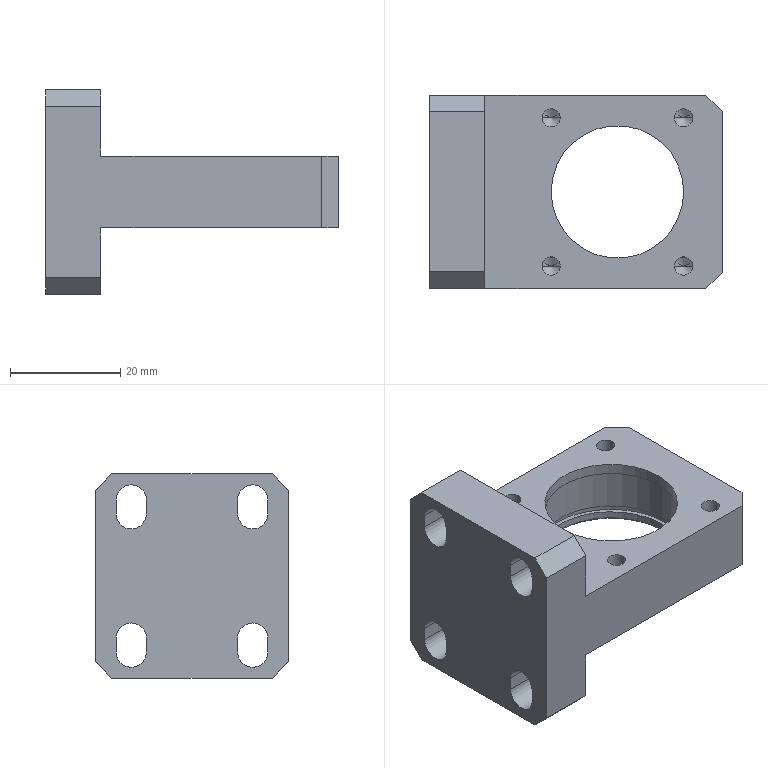Part | NX | features BREP 1 | 1 solid | 65 faces | box 53 x 35 x 37 mm | volume 23524 mm3 | cylinder 28 | plane 27 | cone 10 | commonest cylinder face diameters 5.5 x12 3.3 x8 26 x4 24 x2 27.5 x2